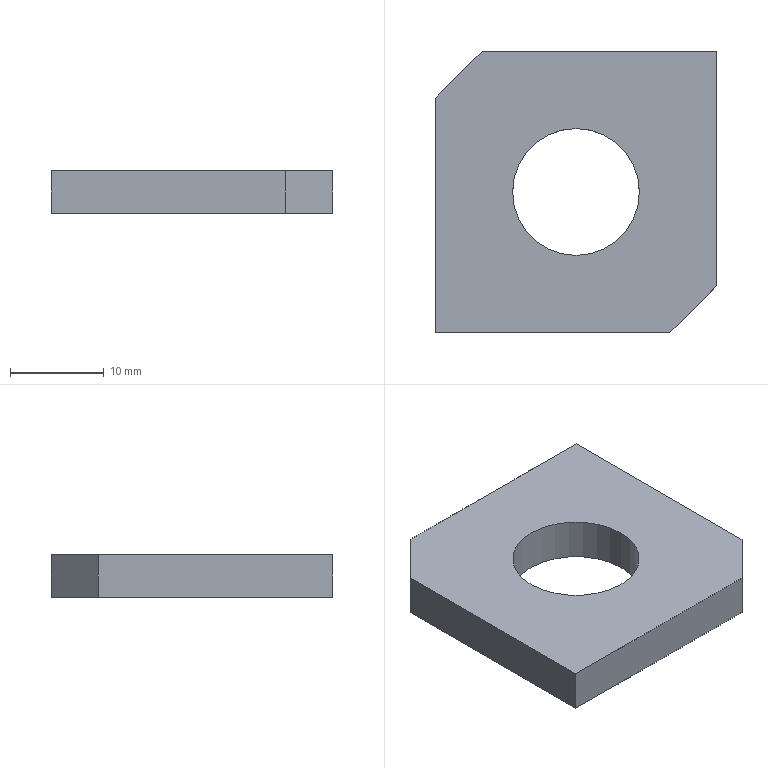Part | SolidWorks | features FlatPattern 1, SMBaseFlange 1, SheetMetal 1 | 1 solid | 10 faces | box 30 x 30 x 4.5 mm | volume 3293 mm3 | plane 8 | cylinder 2 | commonest cylinder face diameters 13.5 x2
STEP:
#1=CARTESIAN_POINT('',(8.25,15.,-4.5));
#2=VERTEX_POINT('',#1);
#3=CARTESIAN_POINT('',(21.75,15.,-4.5));
#4=VERTEX_POINT('',#3);
#5=CARTESIAN_POINT('',(15.,15.,-4.5));
#6=DIRECTION('',(0.,0.,1.));
#7=DIRECTION('',(1.,0.,0.));
#8=AXIS2_PLACEMENT_3D('',#5,#6,#7);
#9=CIRCLE('',#8,6.75);
#10=EDGE_CURVE('',#2,#4,#9,.T.);
#11=ORIENTED_EDGE('',*,*,#10,.F.);
#12=CARTESIAN_POINT('',(8.25,15.,0.));
#13=VERTEX_POINT('',#12);
#14=CARTESIAN_POINT('',(8.25,15.,-4.5));
#15=DIRECTION('',(0.,0.,1.));
#16=VECTOR('',#15,1000.);
#17=LINE('',#14,#16);
#18=EDGE_CURVE('',#2,#13,#17,.T.);
#19=ORIENTED_EDGE('',*,*,#18,.T.);
#20=CARTESIAN_POINT('',(21.75,15.,0.));
#21=VERTEX_POINT('',#20);
#22=CARTESIAN_POINT('',(15.,15.,0.));
#23=DIRECTION('',(0.,0.,1.));
#24=DIRECTION('',(1.,0.,0.));
#25=AXIS2_PLACEMENT_3D('',#22,#23,#24);
#26=CIRCLE('',#25,6.75);
#27=EDGE_CURVE('',#13,#21,#26,.T.);
#28=ORIENTED_EDGE('',*,*,#27,.T.);
#29=CARTESIAN_POINT('',(21.75,15.,-4.5));
#30=DIRECTION('',(0.,0.,1.));
#31=VECTOR('',#30,1000.);
#32=LINE('',#29,#31);
#33=EDGE_CURVE('',#4,#21,#32,.T.);
#34=ORIENTED_EDGE('',*,*,#33,.F.);
#35=EDGE_LOOP('',(#11,#19,#28,#34));
#36=FACE_OUTER_BOUND('',#35,.T.);
#37=CARTESIAN_POINT('',(15.,15.,-4.5));
#38=DIRECTION('',(0.,0.,1.));
#39=DIRECTION('',(1.,0.,0.));
#40=AXIS2_PLACEMENT_3D('',#37,#38,#39);
#41=CYLINDRICAL_SURFACE('',#40,6.75);
#42=ADVANCED_FACE('',(#36),#41,.F.);
#43=CARTESIAN_POINT('',(0.,25.,0.));
#44=VERTEX_POINT('',#43);
#45=CARTESIAN_POINT('',(0.,0.,0.));
#46=VERTEX_POINT('',#45);
#47=CARTESIAN_POINT('',(0.,0.,0.));
#48=DIRECTION('',(0.,-1.,0.));
#49=VECTOR('',#48,1000.);
#50=LINE('',#47,#49);
#51=EDGE_CURVE('',#44,#46,#50,.T.);
#52=ORIENTED_EDGE('',*,*,#51,.F.);
#53=CARTESIAN_POINT('',(0.,25.,-4.5));
#54=VERTEX_POINT('',#53);
#55=CARTESIAN_POINT('',(0.,25.,-4.5));
#56=DIRECTION('',(0.,0.,1.));
#57=VECTOR('',#56,1000.);
#58=LINE('',#55,#57);
#59=EDGE_CURVE('',#54,#44,#58,.T.);
#60=ORIENTED_EDGE('',*,*,#59,.F.);
#61=CARTESIAN_POINT('',(0.,0.,-4.5));
#62=VERTEX_POINT('',#61);
#63=CARTESIAN_POINT('',(0.,0.,-4.5));
#64=DIRECTION('',(0.,-1.,0.));
#65=VECTOR('',#64,1000.);
#66=LINE('',#63,#65);
#67=EDGE_CURVE('',#54,#62,#66,.T.);
#68=ORIENTED_EDGE('',*,*,#67,.T.);
#69=CARTESIAN_POINT('',(0.,0.,-4.5));
#70=DIRECTION('',(0.,0.,1.));
#71=VECTOR('',#70,1000.);
#72=LINE('',#69,#71);
#73=EDGE_CURVE('',#62,#46,#72,.T.);
#74=ORIENTED_EDGE('',*,*,#73,.T.);
#75=EDGE_LOOP('',(#52,#60,#68,#74));
#76=FACE_OUTER_BOUND('',#75,.T.);
#77=CARTESIAN_POINT('',(0.,0.,-4.5));
#78=DIRECTION('',(-1.,0.,0.));
#79=DIRECTION('',(0.,0.,1.));
#80=AXIS2_PLACEMENT_3D('',#77,#78,#79);
#81=PLANE('',#80);
#82=ADVANCED_FACE('',(#76),#81,.T.);
#83=CARTESIAN_POINT('',(5.,30.,0.));
#84=VERTEX_POINT('',#83);
#85=CARTESIAN_POINT('',(0.,25.,0.));
#86=DIRECTION('',(-0.7071,-0.7071,0.));
#87=VECTOR('',#86,1000.);
#88=LINE('',#85,#87);
#89=EDGE_CURVE('',#84,#44,#88,.T.);
#90=ORIENTED_EDGE('',*,*,#89,.F.);
#91=CARTESIAN_POINT('',(5.,30.,-4.5));
#92=VERTEX_POINT('',#91);
#93=CARTESIAN_POINT('',(5.,30.,-4.5));
#94=DIRECTION('',(0.,0.,1.));
#95=VECTOR('',#94,1000.);
#96=LINE('',#93,#95);
#97=EDGE_CURVE('',#92,#84,#96,.T.);
#98=ORIENTED_EDGE('',*,*,#97,.F.);
#99=CARTESIAN_POINT('',(0.,25.,-4.5));
#100=DIRECTION('',(-0.7071,-0.7071,0.));
#101=VECTOR('',#100,1000.);
#102=LINE('',#99,#101);
#103=EDGE_CURVE('',#92,#54,#102,.T.);
#104=ORIENTED_EDGE('',*,*,#103,.T.);
#105=ORIENTED_EDGE('',*,*,#59,.T.);
#106=EDGE_LOOP('',(#90,#98,#104,#105));
#107=FACE_OUTER_BOUND('',#106,.T.);
#108=CARTESIAN_POINT('',(0.,25.,-4.5));
#109=DIRECTION('',(-0.7071,0.7071,0.));
#110=DIRECTION('',(-0.7071,-0.7071,0.));
#111=AXIS2_PLACEMENT_3D('',#108,#109,#110);
#112=PLANE('',#111);
#113=ADVANCED_FACE('',(#107),#112,.T.);
#114=CARTESIAN_POINT('',(30.,30.,0.));
#115=VERTEX_POINT('',#114);
#116=CARTESIAN_POINT('',(5.,30.,0.));
#117=DIRECTION('',(-1.,0.,0.));
#118=VECTOR('',#117,1000.);
#119=LINE('',#116,#118);
#120=EDGE_CURVE('',#115,#84,#119,.T.);
#121=ORIENTED_EDGE('',*,*,#120,.F.);
#122=CARTESIAN_POINT('',(30.,30.,-4.5));
#123=VERTEX_POINT('',#122);
#124=CARTESIAN_POINT('',(30.,30.,-4.5));
#125=DIRECTION('',(0.,0.,1.));
#126=VECTOR('',#125,1000.);
#127=LINE('',#124,#126);
#128=EDGE_CURVE('',#123,#115,#127,.T.);
#129=ORIENTED_EDGE('',*,*,#128,.F.);
#130=CARTESIAN_POINT('',(5.,30.,-4.5));
#131=DIRECTION('',(-1.,0.,0.));
#132=VECTOR('',#131,1000.);
#133=LINE('',#130,#132);
#134=EDGE_CURVE('',#123,#92,#133,.T.);
#135=ORIENTED_EDGE('',*,*,#134,.T.);
#136=ORIENTED_EDGE('',*,*,#97,.T.);
#137=EDGE_LOOP('',(#121,#129,#135,#136));
#138=FACE_OUTER_BOUND('',#137,.T.);
#139=CARTESIAN_POINT('',(5.,30.,-4.5));
#140=DIRECTION('',(0.,1.,0.));
#141=DIRECTION('',(0.,0.,1.));
#142=AXIS2_PLACEMENT_3D('',#139,#140,#141);
#143=PLANE('',#142);
#144=ADVANCED_FACE('',(#138),#143,.T.);
#145=CARTESIAN_POINT('',(30.,5.,0.));
#146=VERTEX_POINT('',#145);
#147=CARTESIAN_POINT('',(30.,5.,0.));
#148=DIRECTION('',(0.,1.,0.));
#149=VECTOR('',#148,1000.);
#150=LINE('',#147,#149);
#151=EDGE_CURVE('',#146,#115,#150,.T.);
#152=ORIENTED_EDGE('',*,*,#151,.F.);
#153=CARTESIAN_POINT('',(30.,5.,-4.5));
#154=VERTEX_POINT('',#153);
#155=CARTESIAN_POINT('',(30.,5.,-4.5));
#156=DIRECTION('',(0.,0.,1.));
#157=VECTOR('',#156,1000.);
#158=LINE('',#155,#157);
#159=EDGE_CURVE('',#154,#146,#158,.T.);
#160=ORIENTED_EDGE('',*,*,#159,.F.);
#161=CARTESIAN_POINT('',(30.,5.,-4.5));
#162=DIRECTION('',(0.,1.,0.));
#163=VECTOR('',#162,1000.);
#164=LINE('',#161,#163);
#165=EDGE_CURVE('',#154,#123,#164,.T.);
#166=ORIENTED_EDGE('',*,*,#165,.T.);
#167=ORIENTED_EDGE('',*,*,#128,.T.);
#168=EDGE_LOOP('',(#152,#160,#166,#167));
#169=FACE_OUTER_BOUND('',#168,.T.);
#170=CARTESIAN_POINT('',(30.,5.,-4.5));
#171=DIRECTION('',(1.,0.,0.));
#172=DIRECTION('',(0.,0.,-1.));
#173=AXIS2_PLACEMENT_3D('',#170,#171,#172);
#174=PLANE('',#173);
#175=ADVANCED_FACE('',(#169),#174,.T.);
#176=CARTESIAN_POINT('',(25.,0.,0.));
#177=VERTEX_POINT('',#176);
#178=CARTESIAN_POINT('',(25.,0.,0.));
#179=DIRECTION('',(0.7071,0.7071,0.));
#180=VECTOR('',#179,1000.);
#181=LINE('',#178,#180);
#182=EDGE_CURVE('',#177,#146,#181,.T.);
#183=ORIENTED_EDGE('',*,*,#182,.F.);
#184=CARTESIAN_POINT('',(25.,0.,-4.5));
#185=VERTEX_POINT('',#184);
#186=CARTESIAN_POINT('',(25.,0.,-4.5));
#187=DIRECTION('',(0.,0.,1.));
#188=VECTOR('',#187,1000.);
#189=LINE('',#186,#188);
#190=EDGE_CURVE('',#185,#177,#189,.T.);
#191=ORIENTED_EDGE('',*,*,#190,.F.);
#192=CARTESIAN_POINT('',(25.,0.,-4.5));
#193=DIRECTION('',(0.7071,0.7071,0.));
#194=VECTOR('',#193,1000.);
#195=LINE('',#192,#194);
#196=EDGE_CURVE('',#185,#154,#195,.T.);
#197=ORIENTED_EDGE('',*,*,#196,.T.);
#198=ORIENTED_EDGE('',*,*,#159,.T.);
#199=EDGE_LOOP('',(#183,#191,#197,#198));
#200=FACE_OUTER_BOUND('',#199,.T.);
#201=CARTESIAN_POINT('',(25.,0.,-4.5));
#202=DIRECTION('',(0.7071,-0.7071,0.));
#203=DIRECTION('',(0.7071,0.7071,0.));
#204=AXIS2_PLACEMENT_3D('',#201,#202,#203);
#205=PLANE('',#204);
#206=ADVANCED_FACE('',(#200),#205,.T.);
#207=CARTESIAN_POINT('',(0.,0.,0.));
#208=DIRECTION('',(1.,0.,0.));
#209=VECTOR('',#208,1000.);
#210=LINE('',#207,#209);
#211=EDGE_CURVE('',#46,#177,#210,.T.);
#212=ORIENTED_EDGE('',*,*,#211,.F.);
#213=ORIENTED_EDGE('',*,*,#73,.F.);
#214=CARTESIAN_POINT('',(0.,0.,-4.5));
#215=DIRECTION('',(1.,0.,0.));
#216=VECTOR('',#215,1000.);
#217=LINE('',#214,#216);
#218=EDGE_CURVE('',#62,#185,#217,.T.);
#219=ORIENTED_EDGE('',*,*,#218,.T.);
#220=ORIENTED_EDGE('',*,*,#190,.T.);
#221=EDGE_LOOP('',(#212,#213,#219,#220));
#222=FACE_OUTER_BOUND('',#221,.T.);
#223=CARTESIAN_POINT('',(0.,0.,-4.5));
#224=DIRECTION('',(0.,-1.,0.));
#225=DIRECTION('',(0.,0.,-1.));
#226=AXIS2_PLACEMENT_3D('',#223,#224,#225);
#227=PLANE('',#226);
#228=ADVANCED_FACE('',(#222),#227,.T.);
#229=CARTESIAN_POINT('',(15.,15.,-4.5));
#230=DIRECTION('',(0.,0.,1.));
#231=DIRECTION('',(1.,0.,0.));
#232=AXIS2_PLACEMENT_3D('',#229,#230,#231);
#233=CIRCLE('',#232,6.75);
#234=EDGE_CURVE('',#4,#2,#233,.T.);
#235=ORIENTED_EDGE('',*,*,#234,.T.);
#236=ORIENTED_EDGE('',*,*,#10,.T.);
#237=EDGE_LOOP('',(#235,#236));
#238=FACE_BOUND('',#237,.T.);
#239=ORIENTED_EDGE('',*,*,#67,.F.);
#240=ORIENTED_EDGE('',*,*,#103,.F.);
#241=ORIENTED_EDGE('',*,*,#134,.F.);
#242=ORIENTED_EDGE('',*,*,#165,.F.);
#243=ORIENTED_EDGE('',*,*,#196,.F.);
#244=ORIENTED_EDGE('',*,*,#218,.F.);
#245=EDGE_LOOP('',(#239,#240,#241,#242,#243,#244));
#246=FACE_OUTER_BOUND('',#245,.T.);
#247=CARTESIAN_POINT('',(0.,0.,-4.5));
#248=DIRECTION('',(0.,0.,-1.));
#249=DIRECTION('',(-1.,0.,0.));
#250=AXIS2_PLACEMENT_3D('',#247,#248,#249);
#251=PLANE('',#250);
#252=ADVANCED_FACE('',(#238,#246),#251,.T.);
#253=CARTESIAN_POINT('',(15.,15.,0.));
#254=DIRECTION('',(0.,0.,1.));
#255=DIRECTION('',(1.,0.,0.));
#256=AXIS2_PLACEMENT_3D('',#253,#254,#255);
#257=CIRCLE('',#256,6.75);
#258=EDGE_CURVE('',#21,#13,#257,.T.);
#259=ORIENTED_EDGE('',*,*,#258,.F.);
#260=ORIENTED_EDGE('',*,*,#27,.F.);
#261=EDGE_LOOP('',(#259,#260));
#262=FACE_BOUND('',#261,.T.);
#263=ORIENTED_EDGE('',*,*,#51,.T.);
#264=ORIENTED_EDGE('',*,*,#211,.T.);
#265=ORIENTED_EDGE('',*,*,#182,.T.);
#266=ORIENTED_EDGE('',*,*,#151,.T.);
#267=ORIENTED_EDGE('',*,*,#120,.T.);
#268=ORIENTED_EDGE('',*,*,#89,.T.);
#269=EDGE_LOOP('',(#263,#264,#265,#266,#267,#268));
#270=FACE_OUTER_BOUND('',#269,.T.);
#271=CARTESIAN_POINT('',(0.,0.,0.));
#272=DIRECTION('',(0.,0.,-1.));
#273=DIRECTION('',(-1.,0.,0.));
#274=AXIS2_PLACEMENT_3D('',#271,#272,#273);
#275=PLANE('',#274);
#276=ADVANCED_FACE('',(#262,#270),#275,.F.);
#277=ORIENTED_EDGE('',*,*,#18,.F.);
#278=ORIENTED_EDGE('',*,*,#234,.F.);
#279=ORIENTED_EDGE('',*,*,#33,.T.);
#280=ORIENTED_EDGE('',*,*,#258,.T.);
#281=EDGE_LOOP('',(#277,#278,#279,#280));
#282=FACE_OUTER_BOUND('',#281,.T.);
#283=CARTESIAN_POINT('',(15.,15.,-4.5));
#284=DIRECTION('',(0.,0.,1.));
#285=DIRECTION('',(1.,0.,0.));
#286=AXIS2_PLACEMENT_3D('',#283,#284,#285);
#287=CYLINDRICAL_SURFACE('',#286,6.75);
#288=ADVANCED_FACE('',(#282),#287,.F.);
#289=CLOSED_SHELL('',(#42,#82,#113,#144,#175,#206,#228,#252,#276,#288));
#290=MANIFOLD_SOLID_BREP('',#289);
#291=CARTESIAN_POINT('',(0.,0.,0.));
#292=DIRECTION('',(0.,0.,1.));
#293=DIRECTION('',(1.,0.,0.));
#294=AXIS2_PLACEMENT_3D('',#291,#292,#293);
#295=(LENGTH_UNIT()NAMED_UNIT(*)SI_UNIT(.MILLI.,.METRE.));
#296=UNCERTAINTY_MEASURE_WITH_UNIT(LENGTH_MEASURE(0.00001),#295,'','');
#297=(NAMED_UNIT(*)PLANE_ANGLE_UNIT()SI_UNIT($,.RADIAN.));
#298=(NAMED_UNIT(*)SI_UNIT($,.STERADIAN.)SOLID_ANGLE_UNIT());
#299=(GEOMETRIC_REPRESENTATION_CONTEXT(3)GLOBAL_UNCERTAINTY_ASSIGNED_CONTEXT((#296))GLOBAL_UNIT_ASSIGNED_CONTEXT((#295,#297,#298))REPRESENTATION_CONTEXT('',''));
#300=ADVANCED_BREP_SHAPE_REPRESENTATION('',(#290,#294),#299);